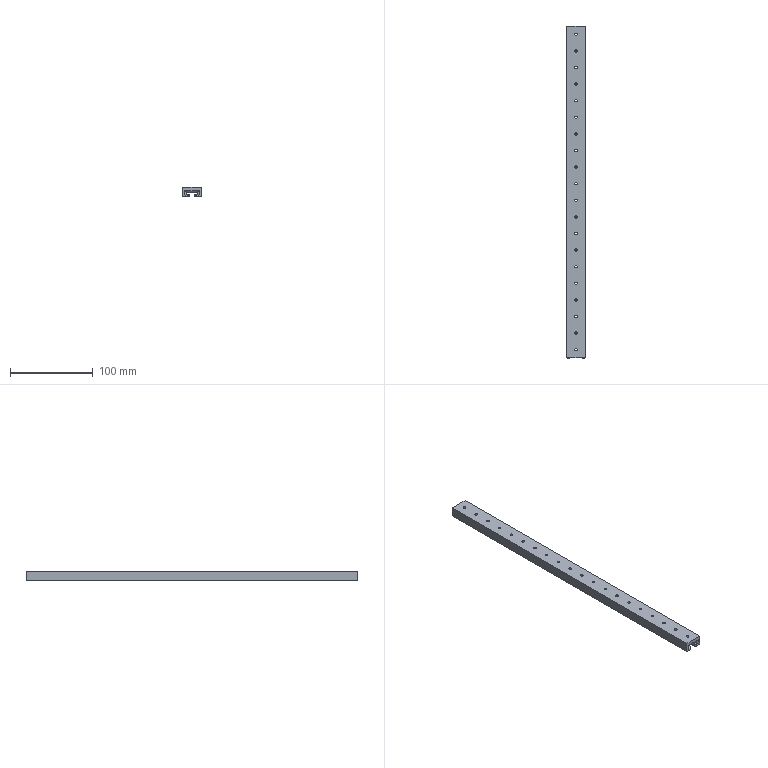Part | SolidWorks | features BaseBody 1 | 1 solid | 171 faces | box 22 x 400 x 12 mm | volume 79490 mm3 | cylinder 93 | cone 40 | plane 38 | commonest cylinder face diameters 3.1 x40 5.7 x40 4 x13